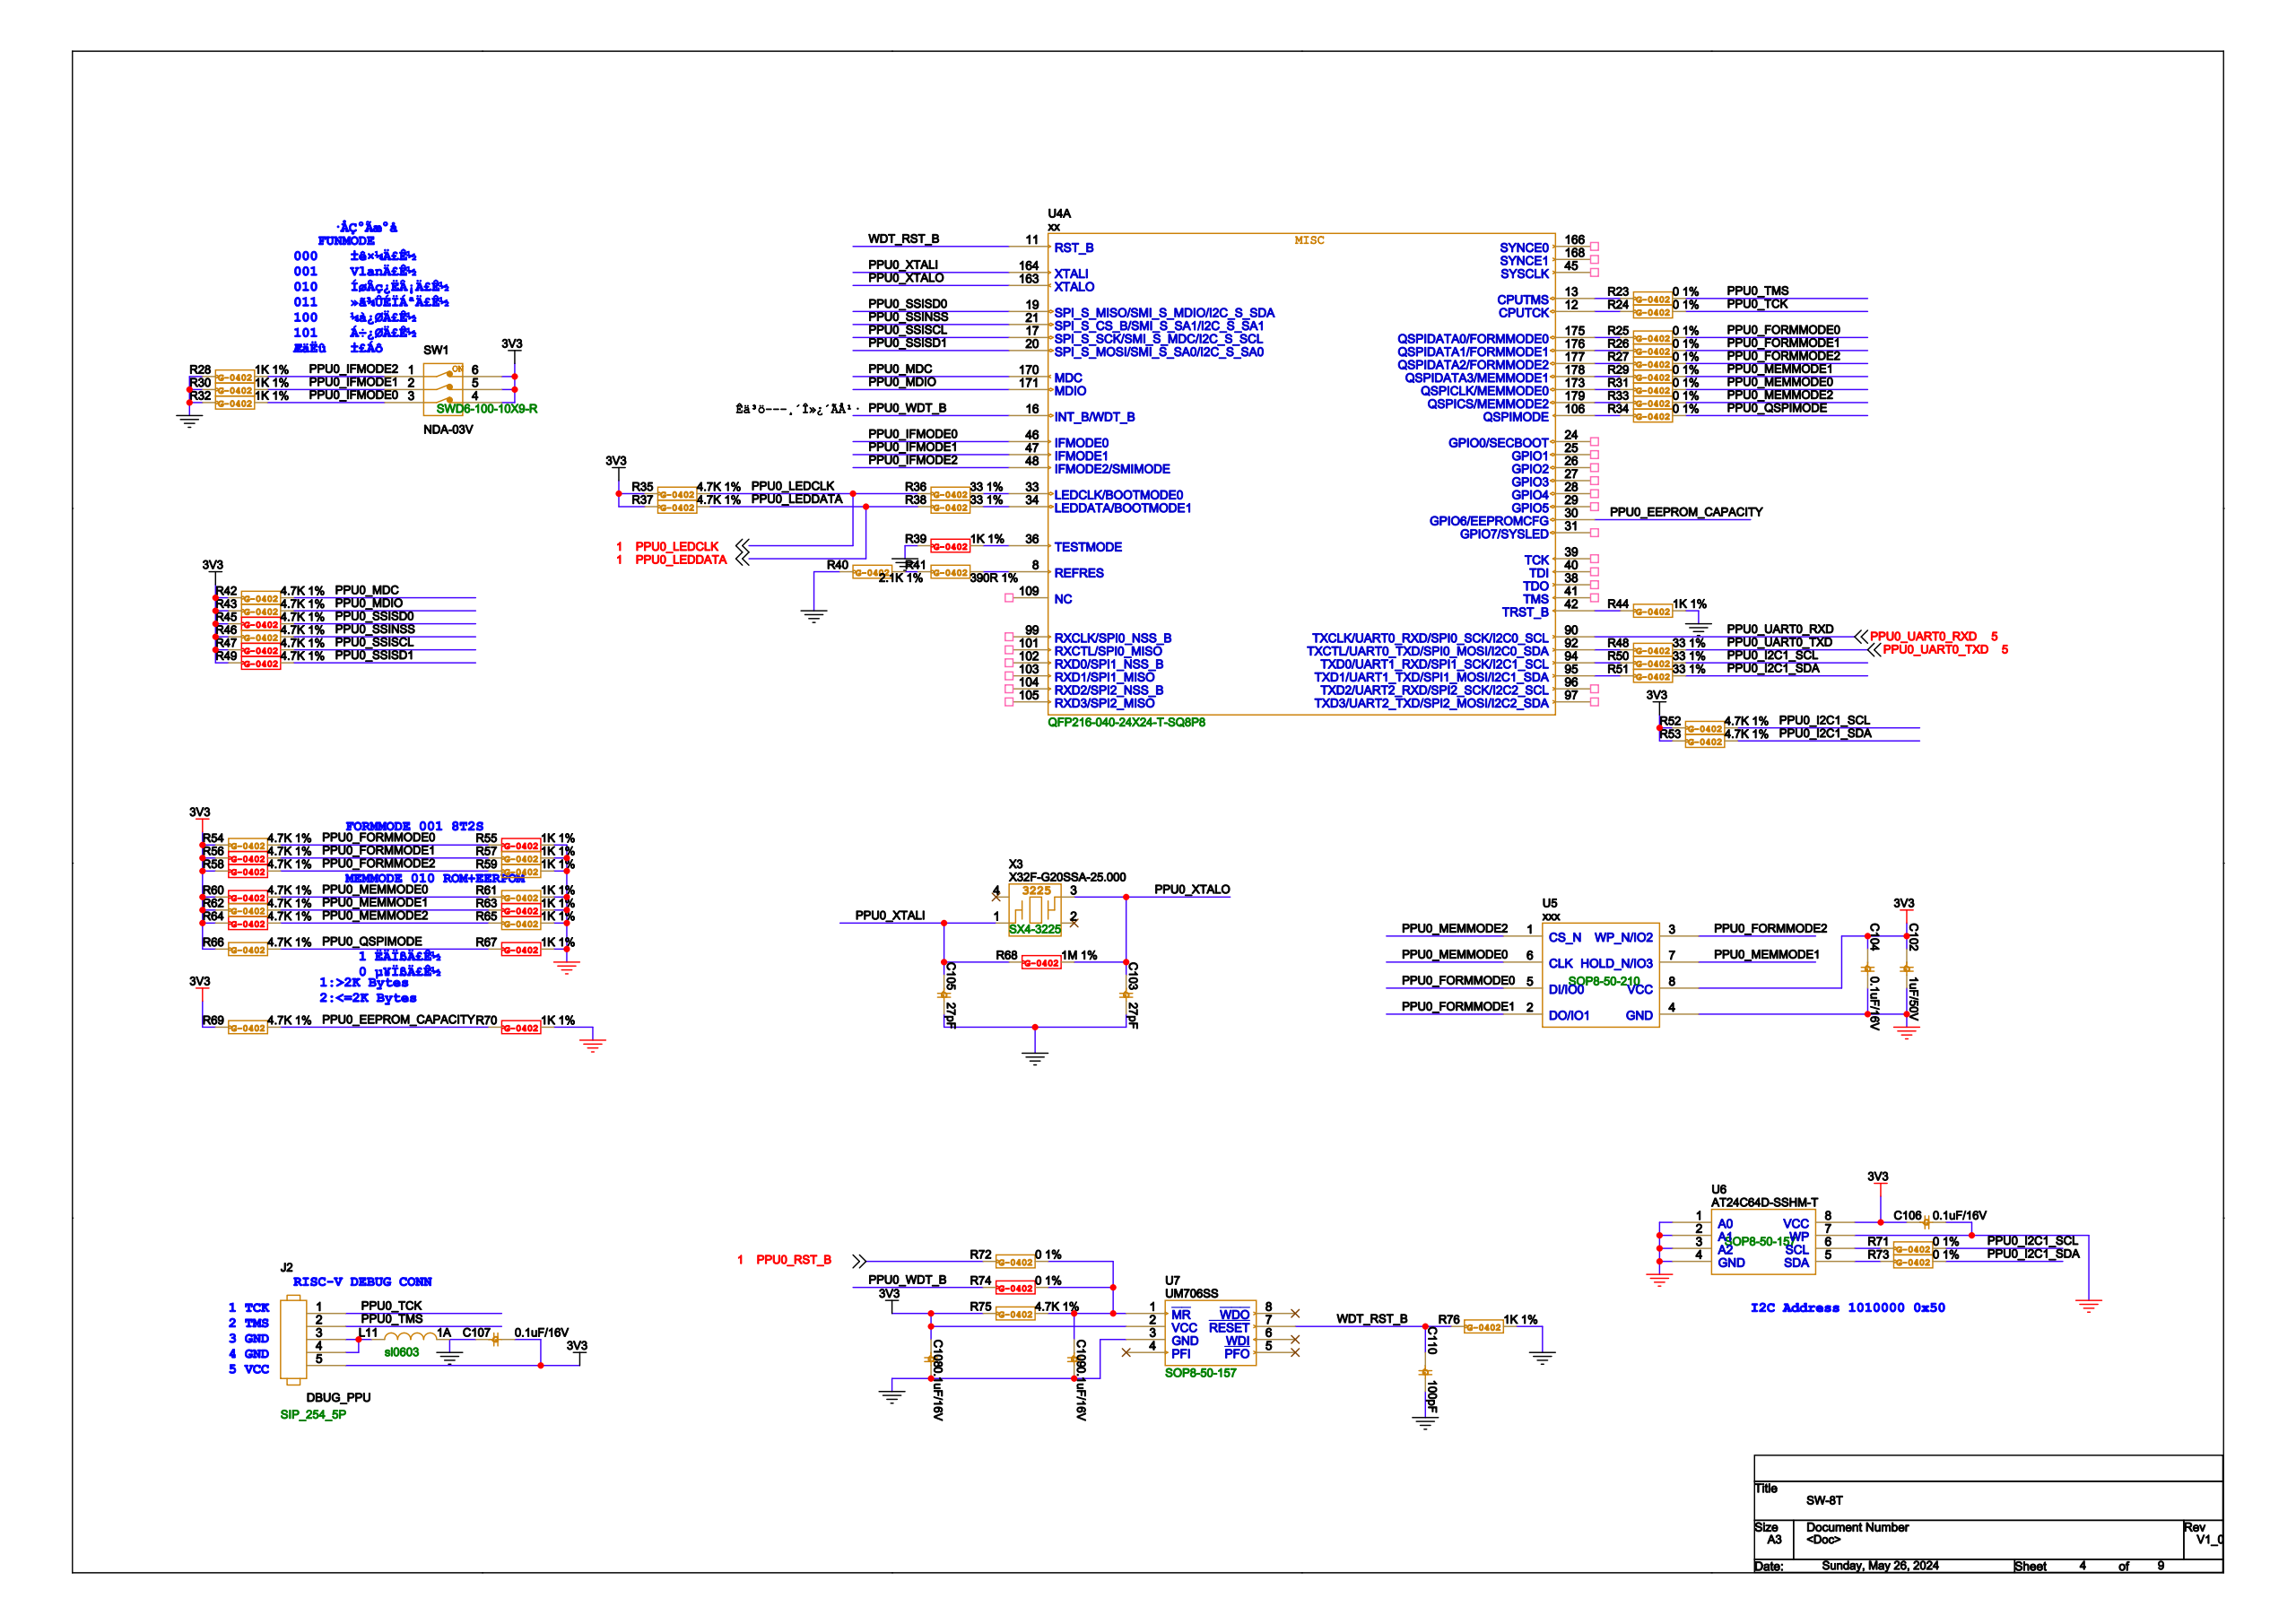Circuit board | Cadence Allegro | 399 parts | 387 nets | one sheet of the schematic
Parts on this sheet (reference | value | footprint):
C102 | 1uF/50V | SC0603
C103 | 27pF | SC0402
C104 | 0.1uF/16V | SC0402
C105 | 27pF | SC0402
C106 | 0.1uF/16V | SC0402
C107 | 0.1uF/16V | SC0402
C110 | 100pF | SC0402
J2 | DBUG_PPU | SIP_254_5P
L11 | 1A | SL0603
R23 | 0 1% | SR0402
R24 | 0 1% | SR0402
R25 | 0 1% | SR0402
R26 | 0 1% | SR0402
R27 | 0 1% | SR0402
R28 | 1K 1% | SR0402
R29 | 0 1% | SR0402
R30 | 1K 1% | SR0402
R31 | 0 1% | SR0402
R32 | 1K 1% | SR0402
R33 | 0 1% | SR0402
R34 | 0 1% | SR0402
R35 | 4.7K 1% | SR0402
R36 | 33 1% | SR0402
R37 | 4.7K 1% | SR0402
R38 | 33 1% | SR0402
R39 | 1K 1% | SR0402
R40 | 2.1K 1% | SR0402
R41 | 390R 1% | SR0402
R42 | 4.7K 1% | SR0402
R43 | 4.7K 1% | SR0402
R44 | 1K 1% | SR0402
R45 | 4.7K 1% | SR0402
R46 | 4.7K 1% | SR0402
R47 | 4.7K 1% | SR0402
R48 | 33 1% | SR0402
R49 | 4.7K 1% | SR0402
R50 | 33 1% | SR0402
R51 | 33 1% | SR0402
R52 | 4.7K 1% | SR0402
R53 | 4.7K 1% | SR0402
R54 | 4.7K 1% | SR0402
R55 | 1K 1% | SR0402
R56 | 4.7K 1% | SR0402
R57 | 1K 1% | SR0402
R58 | 4.7K 1% | SR0402
R59 | 1K 1% | SR0402
R60 | 4.7K 1% | SR0402
R61 | 1K 1% | SR0402
R62 | 4.7K 1% | SR0402
R63 | 1K 1% | SR0402
R64 | 4.7K 1% | SR0402
R65 | 1K 1% | SR0402
R66 | 4.7K 1% | SR0402
R67 | 1K 1% | SR0402
R68 | 1M 1% | SR0402
R69 | 4.7K 1% | SR0402
R70 | 1K 1% | SR0402
R71 | 0 1% | SR0402
R72 | 0 1% | SR0402
R73 | 0 1% | SR0402
R74 | 0 1% | SR0402
R75 | 4.7K 1% | SR0402
R76 | 1K 1% | SR0402
SW1 | NDA-03V | SWD6-100-10X9-R
U4 | xx | QFP216-040-24X24-T-SQ8P8
U5 | xxx | SOP8-50-210
U6 | AT24C64D-SSHM-T | SOP8-50-157
U7 | UM706SS | SOP8-50-157
X3 | X32F-G20SSA-25.000 | SX4-3225
Nets of these parts (net: part-pin ...):
GND: C102-2 C103-2 C104-2 C105-2 C106-2 C107-1 C110-2 L11-2 R28-1 R30-1 R32-1 R39-1 R40-1 R44-2 R55-2 R57-2 R59-2 R61-2 R63-2 R65-2 R67-2 R70-2 R76-2 U5-4 U6-1 U6-2 U6-3 U6-4 U6-7 U7-3 U4-7
PPU0_UART0_RXD: U4-90
PPU0_UART0_TXD: R48-2
3V3: C102-1 C104-1 C106-1 C107-2 J2-5 R35-1 R37-1 R42-1 R43-1 R45-1 R46-1 R47-1 R49-1 R52-1 R53-1 R54-1 R56-1 R58-1 R60-1 R62-1 R64-1 R66-1 R69-1 R75-1 SW1-4 SW1-5 SW1-6 U5-8 U6-8 U7-2
N17699332: R72-2 R74-2 R75-2 U7-1
PPU0_XTALO: C103-1 R68-2 X3-3 U4-163
PPU0_XTALI: C105-1 R68-1 X3-1 U4-164
WDT_RST_B: C110-1 R76-1 U7-7 U4-11
PPU0_TCK: J2-1 R24-2
PPU0_TMS: J2-2 R23-2
N17698788: J2-3 J2-4 L11-1
N17699436: R23-1 U4-13
N17699431: R24-1 U4-12
N17698978: R25-1 U4-175
PPU0_FORMMODE0: R25-2 R54-2 R55-1 U5-5
N17698980: R26-1 U4-176
PPU0_FORMMODE1: R26-2 R56-2 R57-1 U5-2
N17699006: R27-1 U4-177
PPU0_FORMMODE2: R27-2 R58-2 R59-1 U5-3
N17699016: R29-1 U4-178
PPU0_MEMMODE1: R29-2 R62-2 R63-1 U5-7
N17699026: R31-1 U4-173
PPU0_MEMMODE0: R31-2 R60-2 R61-1 U5-6
N17699036: R33-1 U4-179
PPU0_MEMMODE2: R33-2 R64-2 R65-1 U5-1
N17699062: R34-1 U4-106
PPU0_QSPIMODE: R34-2 R66-2 R67-1
N17700565: R71-1 U6-6
PPU0_I2C1_SCL: R50-2 R52-2 R71-2
PPU0_RST_B: R72-1
N17700575: R73-1 U6-5
PPU0_I2C1_SDA: R51-2 R53-2 R73-2
PPU0_WDT_B: R74-1 U4-16
PPU0_IFMODE2: R28-2 SW1-1 U4-48
PPU0_IFMODE1: R30-2 SW1-2 U4-47
PPU0_IFMODE0: R32-2 SW1-3 U4-46
N17699050: R39-2 U4-36
N17698861: R44-1 U4-42
PPU0_EEPROM_CAPACITY: R69-2 R70-1 U4-30
PPU0_LEDCLK: R35-2 R36-1
PPU0_LEDDATA: R37-2 R38-1
PPU0_MDC: R42-2 U4-170
PPU0_MDIO: R43-2 U4-171
PPU0_SSISD0: R45-2 U4-19
PPU0_SSINSS: R46-2 U4-21
PPU0_SSISCL: R47-2 U4-17
PPU0_SSISD1: R49-2 U4-20
N17698855: R36-2 U4-33
N17698857: R38-2 U4-34
N17699087: R48-1 U4-92
N17699100: R50-1 U4-94
N17699113: R51-1 U4-95
N17836965: R40-2 R41-1
N17698859: R41-2 U4-8